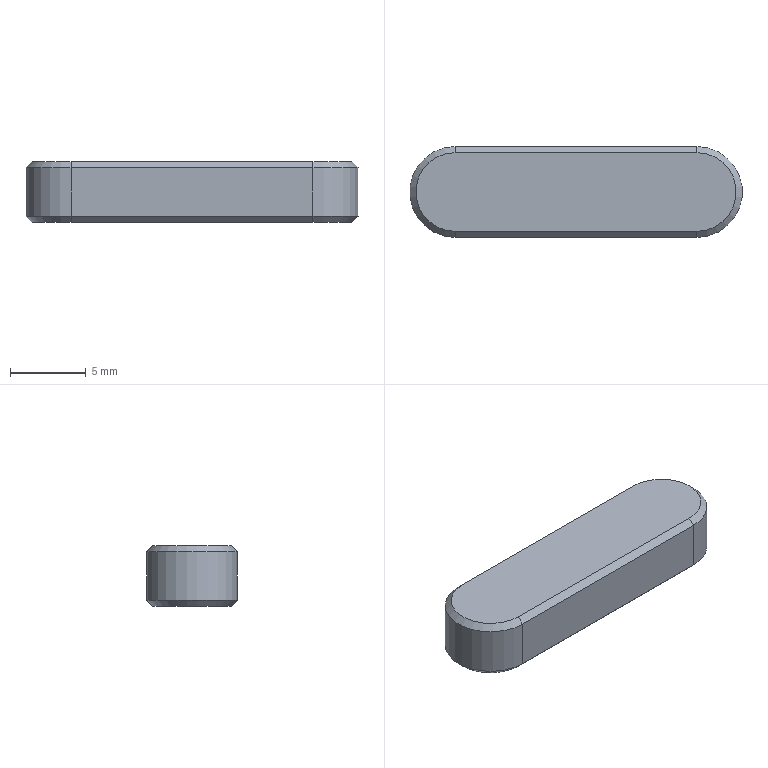Part | SolidWorks | features BaseBody 1 | 1 solid | 14 faces | box 22 x 6 x 4 mm | volume 489.095 mm3 | plane 8 | cone 4 | cylinder 2 | commonest cylinder face diameters 6 x2
STEP:
#1=CARTESIAN_POINT('',(19.,-2.6,-2.5));
#2=VERTEX_POINT('',#1);
#3=CARTESIAN_POINT('',(19.,-3.,-2.1));
#4=VERTEX_POINT('',#3);
#5=CARTESIAN_POINT('',(19.,-2.6,-2.5));
#6=DIRECTION('',(0.,-0.7071,0.7071));
#7=VECTOR('',#6,1000.);
#8=LINE('',#5,#7);
#9=EDGE_CURVE('',#2,#4,#8,.T.);
#10=ORIENTED_EDGE('',*,*,#9,.T.);
#11=CARTESIAN_POINT('',(3.,-3.,-2.1));
#12=VERTEX_POINT('',#11);
#13=CARTESIAN_POINT('',(7.,-3.,-2.1));
#14=DIRECTION('',(-1.,0.,0.));
#15=VECTOR('',#14,1000.);
#16=LINE('',#13,#15);
#17=EDGE_CURVE('',#4,#12,#16,.T.);
#18=ORIENTED_EDGE('',*,*,#17,.T.);
#19=CARTESIAN_POINT('',(3.,-2.6,-2.5));
#20=VERTEX_POINT('',#19);
#21=CARTESIAN_POINT('',(3.,-3.,-2.1));
#22=DIRECTION('',(0.,0.7071,-0.7071));
#23=VECTOR('',#22,1000.);
#24=LINE('',#21,#23);
#25=EDGE_CURVE('',#12,#20,#24,.T.);
#26=ORIENTED_EDGE('',*,*,#25,.T.);
#27=CARTESIAN_POINT('',(7.,-2.6,-2.5));
#28=DIRECTION('',(1.,0.,0.));
#29=VECTOR('',#28,1000.);
#30=LINE('',#27,#29);
#31=EDGE_CURVE('',#20,#2,#30,.T.);
#32=ORIENTED_EDGE('',*,*,#31,.T.);
#33=EDGE_LOOP('',(#10,#18,#26,#32));
#34=FACE_OUTER_BOUND('',#33,.T.);
#35=CARTESIAN_POINT('',(7.,-2.8,-2.3));
#36=DIRECTION('',(0.,-0.7071,-0.7071));
#37=DIRECTION('',(0.,0.7071,-0.7071));
#38=AXIS2_PLACEMENT_3D('',#35,#36,#37);
#39=PLANE('',#38);
#40=ADVANCED_FACE('',(#34),#39,.T.);
#41=CARTESIAN_POINT('',(19.,2.6,-2.5));
#42=VERTEX_POINT('',#41);
#43=CARTESIAN_POINT('',(19.,3.,-2.1));
#44=VERTEX_POINT('',#43);
#45=CARTESIAN_POINT('',(19.,2.6,-2.5));
#46=DIRECTION('',(0.,0.7071,0.7071));
#47=VECTOR('',#46,1000.);
#48=LINE('',#45,#47);
#49=EDGE_CURVE('',#42,#44,#48,.T.);
#50=ORIENTED_EDGE('',*,*,#49,.T.);
#51=CARTESIAN_POINT('',(19.,0.,-2.1));
#52=DIRECTION('',(0.,0.,-1.));
#53=DIRECTION('',(0.,1.,0.));
#54=AXIS2_PLACEMENT_3D('',#51,#52,#53);
#55=CIRCLE('',#54,3.);
#56=EDGE_CURVE('',#44,#4,#55,.T.);
#57=ORIENTED_EDGE('',*,*,#56,.T.);
#58=ORIENTED_EDGE('',*,*,#9,.F.);
#59=CARTESIAN_POINT('',(19.,0.,-2.5));
#60=DIRECTION('',(0.,0.,1.));
#61=DIRECTION('',(0.,1.,0.));
#62=AXIS2_PLACEMENT_3D('',#59,#60,#61);
#63=CIRCLE('',#62,2.6);
#64=EDGE_CURVE('',#2,#42,#63,.T.);
#65=ORIENTED_EDGE('',*,*,#64,.T.);
#66=EDGE_LOOP('',(#50,#57,#58,#65));
#67=FACE_OUTER_BOUND('',#66,.T.);
#68=CARTESIAN_POINT('',(19.,0.,-2.3));
#69=DIRECTION('',(0.,0.,1.));
#70=DIRECTION('',(0.,1.,0.));
#71=AXIS2_PLACEMENT_3D('',#68,#69,#70);
#72=CONICAL_SURFACE('',#71,2.8,0.7854);
#73=ADVANCED_FACE('',(#67),#72,.T.);
#74=CARTESIAN_POINT('',(3.,3.,-2.1));
#75=VERTEX_POINT('',#74);
#76=CARTESIAN_POINT('',(3.,2.6,-2.5));
#77=VERTEX_POINT('',#76);
#78=CARTESIAN_POINT('',(3.,3.,-2.1));
#79=DIRECTION('',(0.,-0.7071,-0.7071));
#80=VECTOR('',#79,1000.);
#81=LINE('',#78,#80);
#82=EDGE_CURVE('',#75,#77,#81,.T.);
#83=ORIENTED_EDGE('',*,*,#82,.T.);
#84=CARTESIAN_POINT('',(3.,0.,-2.5));
#85=DIRECTION('',(0.,0.,1.));
#86=DIRECTION('',(0.,-1.,0.));
#87=AXIS2_PLACEMENT_3D('',#84,#85,#86);
#88=CIRCLE('',#87,2.6);
#89=EDGE_CURVE('',#77,#20,#88,.T.);
#90=ORIENTED_EDGE('',*,*,#89,.T.);
#91=ORIENTED_EDGE('',*,*,#25,.F.);
#92=CARTESIAN_POINT('',(3.,0.,-2.1));
#93=DIRECTION('',(0.,0.,-1.));
#94=DIRECTION('',(0.,-1.,0.));
#95=AXIS2_PLACEMENT_3D('',#92,#93,#94);
#96=CIRCLE('',#95,3.);
#97=EDGE_CURVE('',#12,#75,#96,.T.);
#98=ORIENTED_EDGE('',*,*,#97,.T.);
#99=EDGE_LOOP('',(#83,#90,#91,#98));
#100=FACE_OUTER_BOUND('',#99,.T.);
#101=CARTESIAN_POINT('',(3.,0.,-2.3));
#102=DIRECTION('',(0.,0.,1.));
#103=DIRECTION('',(0.,-1.,0.));
#104=AXIS2_PLACEMENT_3D('',#101,#102,#103);
#105=CONICAL_SURFACE('',#104,2.8,0.7854);
#106=ADVANCED_FACE('',(#100),#105,.T.);
#107=ORIENTED_EDGE('',*,*,#49,.F.);
#108=CARTESIAN_POINT('',(15.,2.6,-2.5));
#109=DIRECTION('',(-1.,0.,0.));
#110=VECTOR('',#109,1000.);
#111=LINE('',#108,#110);
#112=EDGE_CURVE('',#42,#77,#111,.T.);
#113=ORIENTED_EDGE('',*,*,#112,.T.);
#114=ORIENTED_EDGE('',*,*,#82,.F.);
#115=CARTESIAN_POINT('',(15.,3.,-2.1));
#116=DIRECTION('',(1.,0.,0.));
#117=VECTOR('',#116,1000.);
#118=LINE('',#115,#117);
#119=EDGE_CURVE('',#75,#44,#118,.T.);
#120=ORIENTED_EDGE('',*,*,#119,.T.);
#121=EDGE_LOOP('',(#107,#113,#114,#120));
#122=FACE_OUTER_BOUND('',#121,.T.);
#123=CARTESIAN_POINT('',(15.,2.8,-2.3));
#124=DIRECTION('',(0.,0.7071,-0.7071));
#125=DIRECTION('',(-1.,0.,0.));
#126=AXIS2_PLACEMENT_3D('',#123,#124,#125);
#127=PLANE('',#126);
#128=ADVANCED_FACE('',(#122),#127,.T.);
#129=ORIENTED_EDGE('',*,*,#97,.F.);
#130=CARTESIAN_POINT('',(3.,-3.,1.1));
#131=VERTEX_POINT('',#130);
#132=CARTESIAN_POINT('',(3.,-3.,0.));
#133=DIRECTION('',(0.,0.,-1.));
#134=VECTOR('',#133,1000.);
#135=LINE('',#132,#134);
#136=EDGE_CURVE('',#131,#12,#135,.T.);
#137=ORIENTED_EDGE('',*,*,#136,.F.);
#138=CARTESIAN_POINT('',(3.,3.,1.1));
#139=VERTEX_POINT('',#138);
#140=CARTESIAN_POINT('',(3.,0.,1.1));
#141=DIRECTION('',(0.,0.,1.));
#142=DIRECTION('',(0.,-1.,0.));
#143=AXIS2_PLACEMENT_3D('',#140,#141,#142);
#144=CIRCLE('',#143,3.);
#145=EDGE_CURVE('',#139,#131,#144,.T.);
#146=ORIENTED_EDGE('',*,*,#145,.F.);
#147=CARTESIAN_POINT('',(3.,3.,0.));
#148=DIRECTION('',(0.,0.,1.));
#149=VECTOR('',#148,1000.);
#150=LINE('',#147,#149);
#151=EDGE_CURVE('',#75,#139,#150,.T.);
#152=ORIENTED_EDGE('',*,*,#151,.F.);
#153=EDGE_LOOP('',(#129,#137,#146,#152));
#154=FACE_OUTER_BOUND('',#153,.T.);
#155=CARTESIAN_POINT('',(3.,0.,0.));
#156=DIRECTION('',(0.,0.,1.));
#157=DIRECTION('',(0.,-1.,0.));
#158=AXIS2_PLACEMENT_3D('',#155,#156,#157);
#159=CYLINDRICAL_SURFACE('',#158,3.);
#160=ADVANCED_FACE('',(#154),#159,.T.);
#161=ORIENTED_EDGE('',*,*,#17,.F.);
#162=CARTESIAN_POINT('',(19.,-3.,1.1));
#163=VERTEX_POINT('',#162);
#164=CARTESIAN_POINT('',(19.,-3.,0.));
#165=DIRECTION('',(0.,0.,-1.));
#166=VECTOR('',#165,1000.);
#167=LINE('',#164,#166);
#168=EDGE_CURVE('',#163,#4,#167,.T.);
#169=ORIENTED_EDGE('',*,*,#168,.F.);
#170=CARTESIAN_POINT('',(7.,-3.,1.1));
#171=DIRECTION('',(1.,0.,0.));
#172=VECTOR('',#171,1000.);
#173=LINE('',#170,#172);
#174=EDGE_CURVE('',#131,#163,#173,.T.);
#175=ORIENTED_EDGE('',*,*,#174,.F.);
#176=ORIENTED_EDGE('',*,*,#136,.T.);
#177=EDGE_LOOP('',(#161,#169,#175,#176));
#178=FACE_OUTER_BOUND('',#177,.T.);
#179=CARTESIAN_POINT('',(3.,-3.,0.));
#180=DIRECTION('',(0.,-1.,0.));
#181=DIRECTION('',(0.,0.,-1.));
#182=AXIS2_PLACEMENT_3D('',#179,#180,#181);
#183=PLANE('',#182);
#184=ADVANCED_FACE('',(#178),#183,.T.);
#185=ORIENTED_EDGE('',*,*,#31,.F.);
#186=ORIENTED_EDGE('',*,*,#89,.F.);
#187=ORIENTED_EDGE('',*,*,#112,.F.);
#188=ORIENTED_EDGE('',*,*,#64,.F.);
#189=EDGE_LOOP('',(#185,#186,#187,#188));
#190=FACE_OUTER_BOUND('',#189,.T.);
#191=CARTESIAN_POINT('',(11.,0.,-2.5));
#192=DIRECTION('',(0.,0.,1.));
#193=DIRECTION('',(1.,0.,0.));
#194=AXIS2_PLACEMENT_3D('',#191,#192,#193);
#195=PLANE('',#194);
#196=ADVANCED_FACE('',(#190),#195,.F.);
#197=CARTESIAN_POINT('',(3.,-2.6,1.5));
#198=VERTEX_POINT('',#197);
#199=CARTESIAN_POINT('',(3.,-3.,1.1));
#200=DIRECTION('',(0.,0.7071,0.7071));
#201=VECTOR('',#200,1000.);
#202=LINE('',#199,#201);
#203=EDGE_CURVE('',#131,#198,#202,.T.);
#204=ORIENTED_EDGE('',*,*,#203,.T.);
#205=CARTESIAN_POINT('',(3.,2.6,1.5));
#206=VERTEX_POINT('',#205);
#207=CARTESIAN_POINT('',(3.,0.,1.5));
#208=DIRECTION('',(0.,0.,-1.));
#209=DIRECTION('',(0.,-1.,0.));
#210=AXIS2_PLACEMENT_3D('',#207,#208,#209);
#211=CIRCLE('',#210,2.6);
#212=EDGE_CURVE('',#198,#206,#211,.T.);
#213=ORIENTED_EDGE('',*,*,#212,.T.);
#214=CARTESIAN_POINT('',(3.,2.6,1.5));
#215=DIRECTION('',(0.,0.7071,-0.7071));
#216=VECTOR('',#215,1000.);
#217=LINE('',#214,#216);
#218=EDGE_CURVE('',#206,#139,#217,.T.);
#219=ORIENTED_EDGE('',*,*,#218,.T.);
#220=ORIENTED_EDGE('',*,*,#145,.T.);
#221=EDGE_LOOP('',(#204,#213,#219,#220));
#222=FACE_OUTER_BOUND('',#221,.T.);
#223=CARTESIAN_POINT('',(3.,0.,1.3));
#224=DIRECTION('',(0.,0.,-1.));
#225=DIRECTION('',(0.,-1.,0.));
#226=AXIS2_PLACEMENT_3D('',#223,#224,#225);
#227=CONICAL_SURFACE('',#226,2.8,0.7854);
#228=ADVANCED_FACE('',(#222),#227,.T.);
#229=CARTESIAN_POINT('',(19.,-2.6,1.5));
#230=VERTEX_POINT('',#229);
#231=CARTESIAN_POINT('',(19.,-3.,1.1));
#232=DIRECTION('',(0.,0.7071,0.7071));
#233=VECTOR('',#232,1000.);
#234=LINE('',#231,#233);
#235=EDGE_CURVE('',#163,#230,#234,.T.);
#236=ORIENTED_EDGE('',*,*,#235,.T.);
#237=CARTESIAN_POINT('',(7.,-2.6,1.5));
#238=DIRECTION('',(-1.,0.,0.));
#239=VECTOR('',#238,1000.);
#240=LINE('',#237,#239);
#241=EDGE_CURVE('',#230,#198,#240,.T.);
#242=ORIENTED_EDGE('',*,*,#241,.T.);
#243=ORIENTED_EDGE('',*,*,#203,.F.);
#244=ORIENTED_EDGE('',*,*,#174,.T.);
#245=EDGE_LOOP('',(#236,#242,#243,#244));
#246=FACE_OUTER_BOUND('',#245,.T.);
#247=CARTESIAN_POINT('',(7.,-2.8,1.3));
#248=DIRECTION('',(0.,-0.7071,0.7071));
#249=DIRECTION('',(-1.,0.,0.));
#250=AXIS2_PLACEMENT_3D('',#247,#248,#249);
#251=PLANE('',#250);
#252=ADVANCED_FACE('',(#246),#251,.T.);
#253=CARTESIAN_POINT('',(19.,2.6,1.5));
#254=VERTEX_POINT('',#253);
#255=CARTESIAN_POINT('',(19.,3.,1.1));
#256=VERTEX_POINT('',#255);
#257=CARTESIAN_POINT('',(19.,2.6,1.5));
#258=DIRECTION('',(0.,0.7071,-0.7071));
#259=VECTOR('',#258,1000.);
#260=LINE('',#257,#259);
#261=EDGE_CURVE('',#254,#256,#260,.T.);
#262=ORIENTED_EDGE('',*,*,#261,.T.);
#263=CARTESIAN_POINT('',(15.,3.,1.1));
#264=DIRECTION('',(-1.,0.,0.));
#265=VECTOR('',#264,1000.);
#266=LINE('',#263,#265);
#267=EDGE_CURVE('',#256,#139,#266,.T.);
#268=ORIENTED_EDGE('',*,*,#267,.T.);
#269=ORIENTED_EDGE('',*,*,#218,.F.);
#270=CARTESIAN_POINT('',(15.,2.6,1.5));
#271=DIRECTION('',(1.,0.,0.));
#272=VECTOR('',#271,1000.);
#273=LINE('',#270,#272);
#274=EDGE_CURVE('',#206,#254,#273,.T.);
#275=ORIENTED_EDGE('',*,*,#274,.T.);
#276=EDGE_LOOP('',(#262,#268,#269,#275));
#277=FACE_OUTER_BOUND('',#276,.T.);
#278=CARTESIAN_POINT('',(15.,2.8,1.3));
#279=DIRECTION('',(0.,0.7071,0.7071));
#280=DIRECTION('',(1.,0.,0.));
#281=AXIS2_PLACEMENT_3D('',#278,#279,#280);
#282=PLANE('',#281);
#283=ADVANCED_FACE('',(#277),#282,.T.);
#284=ORIENTED_EDGE('',*,*,#235,.F.);
#285=CARTESIAN_POINT('',(19.,0.,1.1));
#286=DIRECTION('',(0.,0.,1.));
#287=DIRECTION('',(0.,1.,0.));
#288=AXIS2_PLACEMENT_3D('',#285,#286,#287);
#289=CIRCLE('',#288,3.);
#290=EDGE_CURVE('',#163,#256,#289,.T.);
#291=ORIENTED_EDGE('',*,*,#290,.T.);
#292=ORIENTED_EDGE('',*,*,#261,.F.);
#293=CARTESIAN_POINT('',(19.,0.,1.5));
#294=DIRECTION('',(0.,0.,-1.));
#295=DIRECTION('',(0.,1.,0.));
#296=AXIS2_PLACEMENT_3D('',#293,#294,#295);
#297=CIRCLE('',#296,2.6);
#298=EDGE_CURVE('',#254,#230,#297,.T.);
#299=ORIENTED_EDGE('',*,*,#298,.T.);
#300=EDGE_LOOP('',(#284,#291,#292,#299));
#301=FACE_OUTER_BOUND('',#300,.T.);
#302=CARTESIAN_POINT('',(19.,0.,1.3));
#303=DIRECTION('',(0.,0.,-1.));
#304=DIRECTION('',(0.,1.,0.));
#305=AXIS2_PLACEMENT_3D('',#302,#303,#304);
#306=CONICAL_SURFACE('',#305,2.8,0.7854);
#307=ADVANCED_FACE('',(#301),#306,.T.);
#308=ORIENTED_EDGE('',*,*,#212,.F.);
#309=ORIENTED_EDGE('',*,*,#241,.F.);
#310=ORIENTED_EDGE('',*,*,#298,.F.);
#311=ORIENTED_EDGE('',*,*,#274,.F.);
#312=EDGE_LOOP('',(#308,#309,#310,#311));
#313=FACE_OUTER_BOUND('',#312,.T.);
#314=CARTESIAN_POINT('',(11.,0.,1.5));
#315=DIRECTION('',(0.,0.,1.));
#316=DIRECTION('',(1.,0.,0.));
#317=AXIS2_PLACEMENT_3D('',#314,#315,#316);
#318=PLANE('',#317);
#319=ADVANCED_FACE('',(#313),#318,.T.);
#320=ORIENTED_EDGE('',*,*,#119,.F.);
#321=ORIENTED_EDGE('',*,*,#151,.T.);
#322=ORIENTED_EDGE('',*,*,#267,.F.);
#323=CARTESIAN_POINT('',(19.,3.,0.));
#324=DIRECTION('',(0.,0.,-1.));
#325=VECTOR('',#324,1000.);
#326=LINE('',#323,#325);
#327=EDGE_CURVE('',#256,#44,#326,.T.);
#328=ORIENTED_EDGE('',*,*,#327,.T.);
#329=EDGE_LOOP('',(#320,#321,#322,#328));
#330=FACE_OUTER_BOUND('',#329,.T.);
#331=CARTESIAN_POINT('',(19.,3.,0.));
#332=DIRECTION('',(0.,1.,0.));
#333=DIRECTION('',(1.,0.,0.));
#334=AXIS2_PLACEMENT_3D('',#331,#332,#333);
#335=PLANE('',#334);
#336=ADVANCED_FACE('',(#330),#335,.T.);
#337=ORIENTED_EDGE('',*,*,#56,.F.);
#338=ORIENTED_EDGE('',*,*,#327,.F.);
#339=ORIENTED_EDGE('',*,*,#290,.F.);
#340=ORIENTED_EDGE('',*,*,#168,.T.);
#341=EDGE_LOOP('',(#337,#338,#339,#340));
#342=FACE_OUTER_BOUND('',#341,.T.);
#343=CARTESIAN_POINT('',(19.,0.,0.));
#344=DIRECTION('',(0.,0.,1.));
#345=DIRECTION('',(0.,1.,0.));
#346=AXIS2_PLACEMENT_3D('',#343,#344,#345);
#347=CYLINDRICAL_SURFACE('',#346,3.);
#348=ADVANCED_FACE('',(#342),#347,.T.);
#349=CLOSED_SHELL('',(#40,#73,#106,#128,#160,#184,#196,#228,#252,#283,#307,#319,#336,#348));
#350=MANIFOLD_SOLID_BREP('',#349);
#351=CARTESIAN_POINT('',(0.,0.,0.));
#352=DIRECTION('',(0.,0.,1.));
#353=DIRECTION('',(1.,0.,0.));
#354=AXIS2_PLACEMENT_3D('',#351,#352,#353);
#355=(LENGTH_UNIT()NAMED_UNIT(*)SI_UNIT(.MILLI.,.METRE.));
#356=UNCERTAINTY_MEASURE_WITH_UNIT(LENGTH_MEASURE(0.00001),#355,'','');
#357=(NAMED_UNIT(*)PLANE_ANGLE_UNIT()SI_UNIT($,.RADIAN.));
#358=(NAMED_UNIT(*)SI_UNIT($,.STERADIAN.)SOLID_ANGLE_UNIT());
#359=(GEOMETRIC_REPRESENTATION_CONTEXT(3)GLOBAL_UNCERTAINTY_ASSIGNED_CONTEXT((#356))GLOBAL_UNIT_ASSIGNED_CONTEXT((#355,#357,#358))REPRESENTATION_CONTEXT('',''));
#360=ADVANCED_BREP_SHAPE_REPRESENTATION('',(#350,#354),#359);